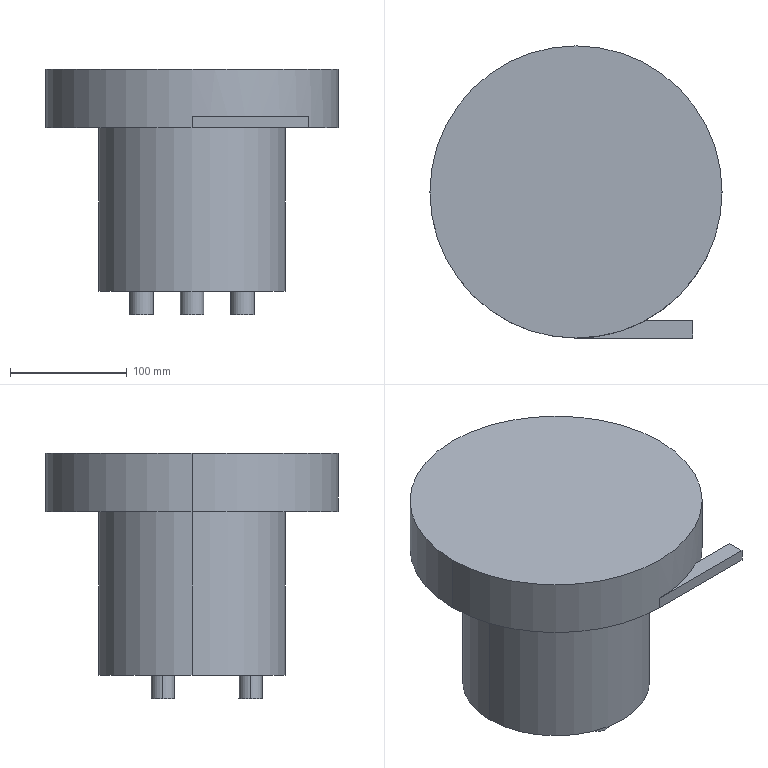Part | STEP file | O-ring vibration plate | 1 solid | 20 faces | box 250 x 250 x 210 mm | volume 5297074 mm3 | cylinder 10 | plane 10 | commonest cylinder face diameters 20 x6 160 x2 250 x2
STEP:
#1=CARTESIAN_POINT('',(0.,0.,0.));
#2=DIRECTION('',(0.,0.,1.));
#3=DIRECTION('',(1.,0.,0.));
#4=AXIS2_PLACEMENT_3D('',#1,#2,#3);
#5=CARTESIAN_POINT('',(33.301,25.,-20.));
#6=VERTEX_POINT('',#5);
#7=CARTESIAN_POINT('',(53.301,25.,-20.));
#8=VERTEX_POINT('',#7);
#9=CARTESIAN_POINT('',(43.301,25.,-20.));
#10=DIRECTION('',(0.,0.,-1.));
#11=DIRECTION('',(0.5,-0.866,0.));
#12=AXIS2_PLACEMENT_3D('',#9,#10,#11);
#13=CIRCLE('',#12,10.);
#14=CARTESIAN_POINT('',(43.301,25.,-20.));
#15=DIRECTION('',(0.,0.,1.));
#16=DIRECTION('',(1.,0.,0.));
#17=AXIS2_PLACEMENT_3D('',#14,#15,#16);
#18=CYLINDRICAL_SURFACE('',#17,10.);
#19=CARTESIAN_POINT('',(5.236,0.));
#20=DIRECTION('',(-1.,0.));
#21=VECTOR('',#20,1.);
#22=LINE('',#19,#21);
#23=(GEOMETRIC_REPRESENTATION_CONTEXT(2)PARAMETRIC_REPRESENTATION_CONTEXT()REPRESENTATION_CONTEXT('',''));
#24=DEFINITIONAL_REPRESENTATION('',(#22),#23);
#25=PCURVE('',#18,#24);
#26=CARTESIAN_POINT('',(43.301,25.,-20.));
#27=DIRECTION('',(0.,0.,-1.));
#28=DIRECTION('',(0.5,-0.866,0.));
#29=AXIS2_PLACEMENT_3D('',#26,#27,#28);
#30=PLANE('',#29);
#31=CARTESIAN_POINT('',(0.,0.));
#32=DIRECTION('',(1.,0.));
#33=AXIS2_PLACEMENT_2D('',#31,#32);
#34=CIRCLE('',#33,10.);
#35=(GEOMETRIC_REPRESENTATION_CONTEXT(2)PARAMETRIC_REPRESENTATION_CONTEXT()REPRESENTATION_CONTEXT('',''));
#36=DEFINITIONAL_REPRESENTATION('',(#34),#35);
#37=PCURVE('',#30,#36);
#38=SURFACE_CURVE('',#13,(#25,#37),.PCURVE_S1.);
#39=EDGE_CURVE('',#6,#8,#38,.T.);
#40=ORIENTED_EDGE('',*,*,#39,.F.);
#41=CARTESIAN_POINT('',(33.301,25.,0.));
#42=VERTEX_POINT('',#41);
#43=CARTESIAN_POINT('',(33.301,25.,-20.));
#44=DIRECTION('',(0.,0.,1.));
#45=VECTOR('',#44,1.);
#46=LINE('',#43,#45);
#47=CARTESIAN_POINT('',(3.142,0.));
#48=DIRECTION('',(0.,1.));
#49=VECTOR('',#48,1.);
#50=LINE('',#47,#49);
#51=(GEOMETRIC_REPRESENTATION_CONTEXT(2)PARAMETRIC_REPRESENTATION_CONTEXT()REPRESENTATION_CONTEXT('',''));
#52=DEFINITIONAL_REPRESENTATION('',(#50),#51);
#53=PCURVE('',#18,#52);
#54=CARTESIAN_POINT('',(43.301,25.,-20.));
#55=DIRECTION('',(0.,0.,1.));
#56=DIRECTION('',(1.,0.,0.));
#57=AXIS2_PLACEMENT_3D('',#54,#55,#56);
#58=CYLINDRICAL_SURFACE('',#57,10.);
#59=CARTESIAN_POINT('',(3.142,0.));
#60=DIRECTION('',(0.,1.));
#61=VECTOR('',#60,1.);
#62=LINE('',#59,#61);
#63=(GEOMETRIC_REPRESENTATION_CONTEXT(2)PARAMETRIC_REPRESENTATION_CONTEXT()REPRESENTATION_CONTEXT('',''));
#64=DEFINITIONAL_REPRESENTATION('',(#62),#63);
#65=PCURVE('',#58,#64);
#66=SURFACE_CURVE('',#46,(#53,#65),.PCURVE_S1.);
#67=EDGE_CURVE('',#6,#42,#66,.T.);
#68=ORIENTED_EDGE('',*,*,#67,.T.);
#69=CARTESIAN_POINT('',(53.301,25.,0.));
#70=VERTEX_POINT('',#69);
#71=CARTESIAN_POINT('',(43.301,25.,0.));
#72=DIRECTION('',(0.,0.,-1.));
#73=DIRECTION('',(1.,0.,0.));
#74=AXIS2_PLACEMENT_3D('',#71,#72,#73);
#75=CIRCLE('',#74,10.);
#76=CARTESIAN_POINT('',(6.283,20.));
#77=DIRECTION('',(-1.,0.));
#78=VECTOR('',#77,1.);
#79=LINE('',#76,#78);
#80=(GEOMETRIC_REPRESENTATION_CONTEXT(2)PARAMETRIC_REPRESENTATION_CONTEXT()REPRESENTATION_CONTEXT('',''));
#81=DEFINITIONAL_REPRESENTATION('',(#79),#80);
#82=PCURVE('',#18,#81);
#83=CARTESIAN_POINT('',(0.,0.,0.));
#84=DIRECTION('',(0.,0.,1.));
#85=DIRECTION('',(1.,0.,0.));
#86=AXIS2_PLACEMENT_3D('',#83,#84,#85);
#87=PLANE('',#86);
#88=CARTESIAN_POINT('',(53.301,25.));
#89=CARTESIAN_POINT('',(53.301,7.679));
#90=CARTESIAN_POINT('',(38.301,16.34));
#91=CARTESIAN_POINT('',(23.301,25.));
#92=CARTESIAN_POINT('',(38.301,33.66));
#93=CARTESIAN_POINT('',(53.301,42.321));
#94=CARTESIAN_POINT('',(53.301,25.));
#95=(BOUNDED_CURVE()B_SPLINE_CURVE(2,(#88,#89,#90,#91,#92,#93,#94),.UNSPECIFIED.,.T.,.F.)B_SPLINE_CURVE_WITH_KNOTS((1,2,2,2,2,1),(-2.094,0.,2.094,4.189,6.283,8.378),.UNSPECIFIED.)CURVE()GEOMETRIC_REPRESENTATION_ITEM()RATIONAL_B_SPLINE_CURVE((1.,0.5,1.,0.5,1.,0.5,1.))REPRESENTATION_ITEM(''));
#96=(GEOMETRIC_REPRESENTATION_CONTEXT(2)PARAMETRIC_REPRESENTATION_CONTEXT()REPRESENTATION_CONTEXT('',''));
#97=DEFINITIONAL_REPRESENTATION('',(#95),#96);
#98=PCURVE('',#87,#97);
#99=SURFACE_CURVE('',#75,(#82,#98),.PCURVE_S1.);
#100=EDGE_CURVE('',#42,#70,#99,.T.);
#101=ORIENTED_EDGE('',*,*,#100,.T.);
#102=CARTESIAN_POINT('',(53.301,25.,-20.));
#103=DIRECTION('',(0.,0.,1.));
#104=VECTOR('',#103,1.);
#105=LINE('',#102,#104);
#106=CARTESIAN_POINT('',(0.,0.));
#107=DIRECTION('',(0.,1.));
#108=VECTOR('',#107,1.);
#109=LINE('',#106,#108);
#110=(GEOMETRIC_REPRESENTATION_CONTEXT(2)PARAMETRIC_REPRESENTATION_CONTEXT()REPRESENTATION_CONTEXT('',''));
#111=DEFINITIONAL_REPRESENTATION('',(#109),#110);
#112=PCURVE('',#18,#111);
#113=CARTESIAN_POINT('',(6.283,0.));
#114=DIRECTION('',(0.,1.));
#115=VECTOR('',#114,1.);
#116=LINE('',#113,#115);
#117=(GEOMETRIC_REPRESENTATION_CONTEXT(2)PARAMETRIC_REPRESENTATION_CONTEXT()REPRESENTATION_CONTEXT('',''));
#118=DEFINITIONAL_REPRESENTATION('',(#116),#117);
#119=PCURVE('',#58,#118);
#120=SURFACE_CURVE('',#105,(#112,#119),.PCURVE_S1.);
#121=EDGE_CURVE('',#8,#70,#120,.T.);
#122=ORIENTED_EDGE('',*,*,#121,.F.);
#123=EDGE_LOOP('',(#40,#68,#101,#122));
#124=FACE_BOUND('',#123,.T.);
#125=ADVANCED_FACE('',(#124),#18,.T.);
#126=CARTESIAN_POINT('',(-53.301,25.,-20.));
#127=VERTEX_POINT('',#126);
#128=CARTESIAN_POINT('',(-33.301,25.,-20.));
#129=VERTEX_POINT('',#128);
#130=CARTESIAN_POINT('',(-43.301,25.,-20.));
#131=DIRECTION('',(0.,0.,-1.));
#132=DIRECTION('',(0.5,0.866,0.));
#133=AXIS2_PLACEMENT_3D('',#130,#131,#132);
#134=CIRCLE('',#133,10.);
#135=CARTESIAN_POINT('',(-43.301,25.,-20.));
#136=DIRECTION('',(0.,0.,1.));
#137=DIRECTION('',(1.,0.,0.));
#138=AXIS2_PLACEMENT_3D('',#135,#136,#137);
#139=CYLINDRICAL_SURFACE('',#138,10.);
#140=CARTESIAN_POINT('',(7.33,0.));
#141=DIRECTION('',(-1.,0.));
#142=VECTOR('',#141,1.);
#143=LINE('',#140,#142);
#144=(GEOMETRIC_REPRESENTATION_CONTEXT(2)PARAMETRIC_REPRESENTATION_CONTEXT()REPRESENTATION_CONTEXT('',''));
#145=DEFINITIONAL_REPRESENTATION('',(#143),#144);
#146=PCURVE('',#139,#145);
#147=CARTESIAN_POINT('',(-43.301,25.,-20.));
#148=DIRECTION('',(0.,0.,-1.));
#149=DIRECTION('',(0.5,0.866,0.));
#150=AXIS2_PLACEMENT_3D('',#147,#148,#149);
#151=PLANE('',#150);
#152=CARTESIAN_POINT('',(0.,0.));
#153=DIRECTION('',(1.,0.));
#154=AXIS2_PLACEMENT_2D('',#152,#153);
#155=CIRCLE('',#154,10.);
#156=(GEOMETRIC_REPRESENTATION_CONTEXT(2)PARAMETRIC_REPRESENTATION_CONTEXT()REPRESENTATION_CONTEXT('',''));
#157=DEFINITIONAL_REPRESENTATION('',(#155),#156);
#158=PCURVE('',#151,#157);
#159=SURFACE_CURVE('',#134,(#146,#158),.PCURVE_S1.);
#160=EDGE_CURVE('',#127,#129,#159,.T.);
#161=ORIENTED_EDGE('',*,*,#160,.F.);
#162=CARTESIAN_POINT('',(-53.301,25.,0.));
#163=VERTEX_POINT('',#162);
#164=CARTESIAN_POINT('',(-53.301,25.,-20.));
#165=DIRECTION('',(0.,0.,1.));
#166=VECTOR('',#165,1.);
#167=LINE('',#164,#166);
#168=CARTESIAN_POINT('',(3.142,0.));
#169=DIRECTION('',(0.,1.));
#170=VECTOR('',#169,1.);
#171=LINE('',#168,#170);
#172=(GEOMETRIC_REPRESENTATION_CONTEXT(2)PARAMETRIC_REPRESENTATION_CONTEXT()REPRESENTATION_CONTEXT('',''));
#173=DEFINITIONAL_REPRESENTATION('',(#171),#172);
#174=PCURVE('',#139,#173);
#175=CARTESIAN_POINT('',(-43.301,25.,-20.));
#176=DIRECTION('',(0.,0.,1.));
#177=DIRECTION('',(1.,0.,0.));
#178=AXIS2_PLACEMENT_3D('',#175,#176,#177);
#179=CYLINDRICAL_SURFACE('',#178,10.);
#180=CARTESIAN_POINT('',(3.142,0.));
#181=DIRECTION('',(0.,1.));
#182=VECTOR('',#181,1.);
#183=LINE('',#180,#182);
#184=(GEOMETRIC_REPRESENTATION_CONTEXT(2)PARAMETRIC_REPRESENTATION_CONTEXT()REPRESENTATION_CONTEXT('',''));
#185=DEFINITIONAL_REPRESENTATION('',(#183),#184);
#186=PCURVE('',#179,#185);
#187=SURFACE_CURVE('',#167,(#174,#186),.PCURVE_S1.);
#188=EDGE_CURVE('',#127,#163,#187,.T.);
#189=ORIENTED_EDGE('',*,*,#188,.T.);
#190=CARTESIAN_POINT('',(-33.301,25.,0.));
#191=VERTEX_POINT('',#190);
#192=CARTESIAN_POINT('',(-43.301,25.,0.));
#193=DIRECTION('',(0.,0.,-1.));
#194=DIRECTION('',(1.,0.,0.));
#195=AXIS2_PLACEMENT_3D('',#192,#193,#194);
#196=CIRCLE('',#195,10.);
#197=CARTESIAN_POINT('',(6.283,20.));
#198=DIRECTION('',(-1.,0.));
#199=VECTOR('',#198,1.);
#200=LINE('',#197,#199);
#201=(GEOMETRIC_REPRESENTATION_CONTEXT(2)PARAMETRIC_REPRESENTATION_CONTEXT()REPRESENTATION_CONTEXT('',''));
#202=DEFINITIONAL_REPRESENTATION('',(#200),#201);
#203=PCURVE('',#139,#202);
#204=CARTESIAN_POINT('',(-33.301,25.));
#205=CARTESIAN_POINT('',(-33.301,7.679));
#206=CARTESIAN_POINT('',(-48.301,16.34));
#207=CARTESIAN_POINT('',(-63.301,25.));
#208=CARTESIAN_POINT('',(-48.301,33.66));
#209=CARTESIAN_POINT('',(-33.301,42.321));
#210=CARTESIAN_POINT('',(-33.301,25.));
#211=(BOUNDED_CURVE()B_SPLINE_CURVE(2,(#204,#205,#206,#207,#208,#209,#210),.UNSPECIFIED.,.T.,.F.)B_SPLINE_CURVE_WITH_KNOTS((1,2,2,2,2,1),(-2.094,0.,2.094,4.189,6.283,8.378),.UNSPECIFIED.)CURVE()GEOMETRIC_REPRESENTATION_ITEM()RATIONAL_B_SPLINE_CURVE((1.,0.5,1.,0.5,1.,0.5,1.))REPRESENTATION_ITEM(''));
#212=(GEOMETRIC_REPRESENTATION_CONTEXT(2)PARAMETRIC_REPRESENTATION_CONTEXT()REPRESENTATION_CONTEXT('',''));
#213=DEFINITIONAL_REPRESENTATION('',(#211),#212);
#214=PCURVE('',#87,#213);
#215=SURFACE_CURVE('',#196,(#203,#214),.PCURVE_S1.);
#216=EDGE_CURVE('',#163,#191,#215,.T.);
#217=ORIENTED_EDGE('',*,*,#216,.T.);
#218=CARTESIAN_POINT('',(-33.301,25.,-20.));
#219=DIRECTION('',(0.,0.,1.));
#220=VECTOR('',#219,1.);
#221=LINE('',#218,#220);
#222=CARTESIAN_POINT('',(0.,0.));
#223=DIRECTION('',(0.,1.));
#224=VECTOR('',#223,1.);
#225=LINE('',#222,#224);
#226=(GEOMETRIC_REPRESENTATION_CONTEXT(2)PARAMETRIC_REPRESENTATION_CONTEXT()REPRESENTATION_CONTEXT('',''));
#227=DEFINITIONAL_REPRESENTATION('',(#225),#226);
#228=PCURVE('',#139,#227);
#229=CARTESIAN_POINT('',(6.283,0.));
#230=DIRECTION('',(0.,1.));
#231=VECTOR('',#230,1.);
#232=LINE('',#229,#231);
#233=(GEOMETRIC_REPRESENTATION_CONTEXT(2)PARAMETRIC_REPRESENTATION_CONTEXT()REPRESENTATION_CONTEXT('',''));
#234=DEFINITIONAL_REPRESENTATION('',(#232),#233);
#235=PCURVE('',#179,#234);
#236=SURFACE_CURVE('',#221,(#228,#235),.PCURVE_S1.);
#237=EDGE_CURVE('',#129,#191,#236,.T.);
#238=ORIENTED_EDGE('',*,*,#237,.F.);
#239=EDGE_LOOP('',(#161,#189,#217,#238));
#240=FACE_BOUND('',#239,.T.);
#241=ADVANCED_FACE('',(#240),#139,.T.);
#242=CARTESIAN_POINT('',(-10.,-50.,-20.));
#243=VERTEX_POINT('',#242);
#244=CARTESIAN_POINT('',(10.,-50.,-20.));
#245=VERTEX_POINT('',#244);
#246=CARTESIAN_POINT('',(0.,-50.,-20.));
#247=DIRECTION('',(0.,0.,-1.));
#248=DIRECTION('',(-1.,0.,0.));
#249=AXIS2_PLACEMENT_3D('',#246,#247,#248);
#250=CIRCLE('',#249,10.);
#251=CARTESIAN_POINT('',(0.,-50.,-20.));
#252=DIRECTION('',(0.,0.,1.));
#253=DIRECTION('',(1.,0.,0.));
#254=AXIS2_PLACEMENT_3D('',#251,#252,#253);
#255=CYLINDRICAL_SURFACE('',#254,10.);
#256=CARTESIAN_POINT('',(3.142,0.));
#257=DIRECTION('',(-1.,0.));
#258=VECTOR('',#257,1.);
#259=LINE('',#256,#258);
#260=(GEOMETRIC_REPRESENTATION_CONTEXT(2)PARAMETRIC_REPRESENTATION_CONTEXT()REPRESENTATION_CONTEXT('',''));
#261=DEFINITIONAL_REPRESENTATION('',(#259),#260);
#262=PCURVE('',#255,#261);
#263=CARTESIAN_POINT('',(0.,-50.,-20.));
#264=DIRECTION('',(0.,0.,-1.));
#265=DIRECTION('',(-1.,0.,0.));
#266=AXIS2_PLACEMENT_3D('',#263,#264,#265);
#267=PLANE('',#266);
#268=CARTESIAN_POINT('',(0.,0.));
#269=DIRECTION('',(1.,0.));
#270=AXIS2_PLACEMENT_2D('',#268,#269);
#271=CIRCLE('',#270,10.);
#272=(GEOMETRIC_REPRESENTATION_CONTEXT(2)PARAMETRIC_REPRESENTATION_CONTEXT()REPRESENTATION_CONTEXT('',''));
#273=DEFINITIONAL_REPRESENTATION('',(#271),#272);
#274=PCURVE('',#267,#273);
#275=SURFACE_CURVE('',#250,(#262,#274),.PCURVE_S1.);
#276=EDGE_CURVE('',#243,#245,#275,.T.);
#277=ORIENTED_EDGE('',*,*,#276,.F.);
#278=CARTESIAN_POINT('',(-10.,-50.,0.));
#279=VERTEX_POINT('',#278);
#280=CARTESIAN_POINT('',(-10.,-50.,-20.));
#281=DIRECTION('',(0.,0.,1.));
#282=VECTOR('',#281,1.);
#283=LINE('',#280,#282);
#284=CARTESIAN_POINT('',(3.142,0.));
#285=DIRECTION('',(0.,1.));
#286=VECTOR('',#285,1.);
#287=LINE('',#284,#286);
#288=(GEOMETRIC_REPRESENTATION_CONTEXT(2)PARAMETRIC_REPRESENTATION_CONTEXT()REPRESENTATION_CONTEXT('',''));
#289=DEFINITIONAL_REPRESENTATION('',(#287),#288);
#290=PCURVE('',#255,#289);
#291=CARTESIAN_POINT('',(0.,-50.,-20.));
#292=DIRECTION('',(0.,0.,1.));
#293=DIRECTION('',(1.,0.,0.));
#294=AXIS2_PLACEMENT_3D('',#291,#292,#293);
#295=CYLINDRICAL_SURFACE('',#294,10.);
#296=CARTESIAN_POINT('',(3.142,0.));
#297=DIRECTION('',(0.,1.));
#298=VECTOR('',#297,1.);
#299=LINE('',#296,#298);
#300=(GEOMETRIC_REPRESENTATION_CONTEXT(2)PARAMETRIC_REPRESENTATION_CONTEXT()REPRESENTATION_CONTEXT('',''));
#301=DEFINITIONAL_REPRESENTATION('',(#299),#300);
#302=PCURVE('',#295,#301);
#303=SURFACE_CURVE('',#283,(#290,#302),.PCURVE_S1.);
#304=EDGE_CURVE('',#243,#279,#303,.T.);
#305=ORIENTED_EDGE('',*,*,#304,.T.);
#306=CARTESIAN_POINT('',(10.,-50.,0.));
#307=VERTEX_POINT('',#306);
#308=CARTESIAN_POINT('',(0.,-50.,0.));
#309=DIRECTION('',(0.,0.,-1.));
#310=DIRECTION('',(1.,0.,0.));
#311=AXIS2_PLACEMENT_3D('',#308,#309,#310);
#312=CIRCLE('',#311,10.);
#313=CARTESIAN_POINT('',(6.283,20.));
#314=DIRECTION('',(-1.,0.));
#315=VECTOR('',#314,1.);
#316=LINE('',#313,#315);
#317=(GEOMETRIC_REPRESENTATION_CONTEXT(2)PARAMETRIC_REPRESENTATION_CONTEXT()REPRESENTATION_CONTEXT('',''));
#318=DEFINITIONAL_REPRESENTATION('',(#316),#317);
#319=PCURVE('',#255,#318);
#320=CARTESIAN_POINT('',(10.,-50.));
#321=CARTESIAN_POINT('',(10.,-67.321));
#322=CARTESIAN_POINT('',(-5.,-58.66));
#323=CARTESIAN_POINT('',(-20.,-50.));
#324=CARTESIAN_POINT('',(-5.,-41.34));
#325=CARTESIAN_POINT('',(10.,-32.679));
#326=CARTESIAN_POINT('',(10.,-50.));
#327=(BOUNDED_CURVE()B_SPLINE_CURVE(2,(#320,#321,#322,#323,#324,#325,#326),.UNSPECIFIED.,.T.,.F.)B_SPLINE_CURVE_WITH_KNOTS((1,2,2,2,2,1),(-2.094,0.,2.094,4.189,6.283,8.378),.UNSPECIFIED.)CURVE()GEOMETRIC_REPRESENTATION_ITEM()RATIONAL_B_SPLINE_CURVE((1.,0.5,1.,0.5,1.,0.5,1.))REPRESENTATION_ITEM(''));
#328=(GEOMETRIC_REPRESENTATION_CONTEXT(2)PARAMETRIC_REPRESENTATION_CONTEXT()REPRESENTATION_CONTEXT('',''));
#329=DEFINITIONAL_REPRESENTATION('',(#327),#328);
#330=PCURVE('',#87,#329);
#331=SURFACE_CURVE('',#312,(#319,#330),.PCURVE_S1.);
#332=EDGE_CURVE('',#279,#307,#331,.T.);
#333=ORIENTED_EDGE('',*,*,#332,.T.);
#334=CARTESIAN_POINT('',(10.,-50.,-20.));
#335=DIRECTION('',(0.,0.,1.));
#336=VECTOR('',#335,1.);
#337=LINE('',#334,#336);
#338=CARTESIAN_POINT('',(0.,0.));
#339=DIRECTION('',(0.,1.));
#340=VECTOR('',#339,1.);
#341=LINE('',#338,#340);
#342=(GEOMETRIC_REPRESENTATION_CONTEXT(2)PARAMETRIC_REPRESENTATION_CONTEXT()REPRESENTATION_CONTEXT('',''));
#343=DEFINITIONAL_REPRESENTATION('',(#341),#342);
#344=PCURVE('',#255,#343);
#345=CARTESIAN_POINT('',(6.283,0.));
#346=DIRECTION('',(0.,1.));
#347=VECTOR('',#346,1.);
#348=LINE('',#345,#347);
#349=(GEOMETRIC_REPRESENTATION_CONTEXT(2)PARAMETRIC_REPRESENTATION_CONTEXT()REPRESENTATION_CONTEXT('',''));
#350=DEFINITIONAL_REPRESENTATION('',(#348),#349);
#351=PCURVE('',#295,#350);
#352=SURFACE_CURVE('',#337,(#344,#351),.PCURVE_S1.);
#353=EDGE_CURVE('',#245,#307,#352,.T.);
#354=ORIENTED_EDGE('',*,*,#353,.F.);
#355=EDGE_LOOP('',(#277,#305,#333,#354));
#356=FACE_BOUND('',#355,.T.);
#357=ADVANCED_FACE('',(#356),#255,.T.);
#358=CARTESIAN_POINT('',(80.,0.,140.));
#359=VERTEX_POINT('',#358);
#360=CARTESIAN_POINT('',(-80.,0.,140.));
#361=VERTEX_POINT('',#360);
#362=CARTESIAN_POINT('',(0.,0.,140.));
#363=DIRECTION('',(0.,0.,1.));
#364=DIRECTION('',(1.,0.,0.));
#365=AXIS2_PLACEMENT_3D('',#362,#363,#364);
#366=CIRCLE('',#365,80.);
#367=CARTESIAN_POINT('',(0.,0.,140.));
#368=DIRECTION('',(0.,0.,-1.));
#369=DIRECTION('',(-1.,0.,0.));
#370=AXIS2_PLACEMENT_3D('',#367,#368,#369);
#371=CYLINDRICAL_SURFACE('',#370,80.);
#372=CARTESIAN_POINT('',(3.142,0.));
#373=DIRECTION('',(-1.,0.));
#374=VECTOR('',#373,1.);
#375=LINE('',#372,#374);
#376=(GEOMETRIC_REPRESENTATION_CONTEXT(2)PARAMETRIC_REPRESENTATION_CONTEXT()REPRESENTATION_CONTEXT('',''));
#377=DEFINITIONAL_REPRESENTATION('',(#375),#376);
#378=PCURVE('',#371,#377);
#379=CARTESIAN_POINT('',(0.,0.,140.));
#380=DIRECTION('',(0.,0.,1.));
#381=DIRECTION('',(1.,0.,0.));
#382=AXIS2_PLACEMENT_3D('',#379,#380,#381);
#383=PLANE('',#382);
#384=CARTESIAN_POINT('',(0.,0.));
#385=DIRECTION('',(1.,0.));
#386=AXIS2_PLACEMENT_2D('',#384,#385);
#387=CIRCLE('',#386,80.);
#388=(GEOMETRIC_REPRESENTATION_CONTEXT(2)PARAMETRIC_REPRESENTATION_CONTEXT()REPRESENTATION_CONTEXT('',''));
#389=DEFINITIONAL_REPRESENTATION('',(#387),#388);
#390=PCURVE('',#383,#389);
#391=SURFACE_CURVE('',#366,(#378,#390),.PCURVE_S1.);
#392=EDGE_CURVE('',#359,#361,#391,.T.);
#393=ORIENTED_EDGE('',*,*,#392,.F.);
#394=CARTESIAN_POINT('',(80.,0.,0.));
#395=VERTEX_POINT('',#394);
#396=CARTESIAN_POINT('',(80.,0.,140.));
#397=DIRECTION('',(0.,0.,-1.));
#398=VECTOR('',#397,1.);
#399=LINE('',#396,#398);
#400=CARTESIAN_POINT('',(3.142,0.));
#401=DIRECTION('',(0.,1.));
#402=VECTOR('',#401,1.);
#403=LINE('',#400,#402);
#404=(GEOMETRIC_REPRESENTATION_CONTEXT(2)PARAMETRIC_REPRESENTATION_CONTEXT()REPRESENTATION_CONTEXT('',''));
#405=DEFINITIONAL_REPRESENTATION('',(#403),#404);
#406=PCURVE('',#371,#405);
#407=CARTESIAN_POINT('',(0.,0.,140.));
#408=DIRECTION('',(0.,0.,-1.));
#409=DIRECTION('',(-1.,0.,0.));
#410=AXIS2_PLACEMENT_3D('',#407,#408,#409);
#411=CYLINDRICAL_SURFACE('',#410,80.);
#412=CARTESIAN_POINT('',(3.142,0.));
#413=DIRECTION('',(0.,1.));
#414=VECTOR('',#413,1.);
#415=LINE('',#412,#414);
#416=(GEOMETRIC_REPRESENTATION_CONTEXT(2)PARAMETRIC_REPRESENTATION_CONTEXT()REPRESENTATION_CONTEXT('',''));
#417=DEFINITIONAL_REPRESENTATION('',(#415),#416);
#418=PCURVE('',#411,#417);
#419=SURFACE_CURVE('',#399,(#406,#418),.PCURVE_S1.);
#420=EDGE_CURVE('',#359,#395,#419,.T.);
#421=ORIENTED_EDGE('',*,*,#420,.T.);
#422=CARTESIAN_POINT('',(-80.,0.,0.));
#423=VERTEX_POINT('',#422);
#424=CARTESIAN_POINT('',(0.,0.,0.));
#425=DIRECTION('',(0.,0.,1.));
#426=DIRECTION('',(1.,0.,0.));
#427=AXIS2_PLACEMENT_3D('',#424,#425,#426);
#428=CIRCLE('',#427,80.);
#429=CARTESIAN_POINT('',(3.142,140.));
#430=DIRECTION('',(-1.,0.));
#431=VECTOR('',#430,1.);
#432=LINE('',#429,#431);
#433=(GEOMETRIC_REPRESENTATION_CONTEXT(2)PARAMETRIC_REPRESENTATION_CONTEXT()REPRESENTATION_CONTEXT('',''));
#434=DEFINITIONAL_REPRESENTATION('',(#432),#433);
#435=PCURVE('',#371,#434);
#436=CARTESIAN_POINT('',(0.,0.));
#437=DIRECTION('',(1.,0.));
#438=AXIS2_PLACEMENT_2D('',#436,#437);
#439=CIRCLE('',#438,80.);
#440=(GEOMETRIC_REPRESENTATION_CONTEXT(2)PARAMETRIC_REPRESENTATION_CONTEXT()REPRESENTATION_CONTEXT('',''));
#441=DEFINITIONAL_REPRESENTATION('',(#439),#440);
#442=PCURVE('',#87,#441);
#443=SURFACE_CURVE('',#428,(#435,#442),.PCURVE_S1.);
#444=EDGE_CURVE('',#395,#423,#443,.T.);
#445=ORIENTED_EDGE('',*,*,#444,.T.);
#446=CARTESIAN_POINT('',(-80.,0.,140.));
#447=DIRECTION('',(0.,0.,-1.));
#448=VECTOR('',#447,1.);
#449=LINE('',#446,#448);
#450=CARTESIAN_POINT('',(0.,0.));
#451=DIRECTION('',(0.,1.));
#452=VECTOR('',#451,1.);
#453=LINE('',#450,#452);
#454=(GEOMETRIC_REPRESENTATION_CONTEXT(2)PARAMETRIC_REPRESENTATION_CONTEXT()REPRESENTATION_CONTEXT('',''));
#455=DEFINITIONAL_REPRESENTATION('',(#453),#454);
#456=PCURVE('',#371,#455);
#457=CARTESIAN_POINT('',(6.283,0.));
#458=DIRECTION('',(0.,1.));
#459=VECTOR('',#458,1.);
#460=LINE('',#457,#459);
#461=(GEOMETRIC_REPRESENTATION_CONTEXT(2)PARAMETRIC_REPRESENTATION_CONTEXT()REPRESENTATION_CONTEXT('',''));
#462=DEFINITIONAL_REPRESENTATION('',(#460),#461);
#463=PCURVE('',#411,#462);
#464=SURFACE_CURVE('',#449,(#456,#463),.PCURVE_S1.);
#465=EDGE_CURVE('',#361,#423,#464,.T.);
#466=ORIENTED_EDGE('',*,*,#465,.F.);
#467=EDGE_LOOP('',(#393,#421,#445,#466));
#468=FACE_BOUND('',#467,.T.);
#469=ADVANCED_FACE('',(#468),#371,.T.);
#470=CARTESIAN_POINT('',(125.,0.,190.));
#471=VERTEX_POINT('',#470);
#472=CARTESIAN_POINT('',(-125.,0.,190.));
#473=VERTEX_POINT('',#472);
#474=CARTESIAN_POINT('',(0.,0.,190.));
#475=DIRECTION('',(0.,0.,1.));
#476=DIRECTION('',(1.,0.,0.));
#477=AXIS2_PLACEMENT_3D('',#474,#475,#476);
#478=CIRCLE('',#477,125.);
#479=CARTESIAN_POINT('',(0.,0.,190.));
#480=DIRECTION('',(0.,0.,-1.));
#481=DIRECTION('',(-1.,0.,0.));
#482=AXIS2_PLACEMENT_3D('',#479,#480,#481);
#483=CYLINDRICAL_SURFACE('',#482,125.);
#484=CARTESIAN_POINT('',(3.142,0.));
#485=DIRECTION('',(-1.,0.));
#486=VECTOR('',#485,1.);
#487=LINE('',#484,#486);
#488=(GEOMETRIC_REPRESENTATION_CONTEXT(2)PARAMETRIC_REPRESENTATION_CONTEXT()REPRESENTATION_CONTEXT('',''));
#489=DEFINITIONAL_REPRESENTATION('',(#487),#488);
#490=PCURVE('',#483,#489);
#491=CARTESIAN_POINT('',(0.,0.,190.));
#492=DIRECTION('',(0.,0.,1.));
#493=DIRECTION('',(1.,0.,0.));
#494=AXIS2_PLACEMENT_3D('',#491,#492,#493);
#495=PLANE('',#494);
#496=CARTESIAN_POINT('',(0.,0.));
#497=DIRECTION('',(1.,0.));
#498=AXIS2_PLACEMENT_2D('',#496,#497);
#499=CIRCLE('',#498,125.);
#500=(GEOMETRIC_REPRESENTATION_CONTEXT(2)PARAMETRIC_REPRESENTATION_CONTEXT()REPRESENTATION_CONTEXT('',''));
#501=DEFINITIONAL_REPRESENTATION('',(#499),#500);
#502=PCURVE('',#495,#501);
#503=SURFACE_CURVE('',#478,(#490,#502),.PCURVE_S1.);
#504=EDGE_CURVE('',#471,#473,#503,.T.);
#505=ORIENTED_EDGE('',*,*,#504,.F.);
#506=CARTESIAN_POINT('',(125.,0.,140.));
#507=VERTEX_POINT('',#506);
#508=CARTESIAN_POINT('',(125.,0.,190.));
#509=DIRECTION('',(0.,0.,-1.));
#510=VECTOR('',#509,1.);
#511=LINE('',#508,#510);
#512=CARTESIAN_POINT('',(3.142,0.));
#513=DIRECTION('',(0.,1.));
#514=VECTOR('',#513,1.);
#515=LINE('',#512,#514);
#516=(GEOMETRIC_REPRESENTATION_CONTEXT(2)PARAMETRIC_REPRESENTATION_CONTEXT()REPRESENTATION_CONTEXT('',''));
#517=DEFINITIONAL_REPRESENTATION('',(#515),#516);
#518=PCURVE('',#483,#517);
#519=CARTESIAN_POINT('',(0.,0.,190.));
#520=DIRECTION('',(0.,0.,-1.));
#521=DIRECTION('',(-1.,0.,0.));
#522=AXIS2_PLACEMENT_3D('',#519,#520,#521);
#523=CYLINDRICAL_SURFACE('',#522,125.);
#524=CARTESIAN_POINT('',(3.142,0.));
#525=DIRECTION('',(0.,1.));
#526=VECTOR('',#525,1.);
#527=LINE('',#524,#526);
#528=(GEOMETRIC_REPRESENTATION_CONTEXT(2)PARAMETRIC_REPRESENTATION_CONTEXT()REPRESENTATION_CONTEXT('',''));
#529=DEFINITIONAL_REPRESENTATION('',(#527),#528);
#530=PCURVE('',#523,#529);
#531=SURFACE_CURVE('',#511,(#518,#530),.PCURVE_S1.);
#532=EDGE_CURVE('',#471,#507,#531,.T.);
#533=ORIENTED_EDGE('',*,*,#532,.T.);
#534=CARTESIAN_POINT('',(-125.,0.,140.));
#535=VERTEX_POINT('',#534);
#536=CARTESIAN_POINT('',(0.,0.,140.));
#537=DIRECTION('',(0.,0.,1.));
#538=DIRECTION('',(1.,0.,0.));
#539=AXIS2_PLACEMENT_3D('',#536,#537,#538);
#540=CIRCLE('',#539,125.);
#541=CARTESIAN_POINT('',(3.142,50.));
#542=DIRECTION('',(-1.,0.));
#543=VECTOR('',#542,1.);
#544=LINE('',#541,#543);
#545=(GEOMETRIC_REPRESENTATION_CONTEXT(2)PARAMETRIC_REPRESENTATION_CONTEXT()REPRESENTATION_CONTEXT('',''));
#546=DEFINITIONAL_REPRESENTATION('',(#544),#545);
#547=PCURVE('',#483,#546);
#548=CARTESIAN_POINT('',(0.,0.));
#549=DIRECTION('',(1.,0.));
#550=AXIS2_PLACEMENT_2D('',#548,#549);
#551=CIRCLE('',#550,125.);
#552=(GEOMETRIC_REPRESENTATION_CONTEXT(2)PARAMETRIC_REPRESENTATION_CONTEXT()REPRESENTATION_CONTEXT('',''));
#553=DEFINITIONAL_REPRESENTATION('',(#551),#552);
#554=PCURVE('',#383,#553);
#555=SURFACE_CURVE('',#540,(#547,#554),.PCURVE_S1.);
#556=EDGE_CURVE('',#507,#535,#555,.T.);
#557=ORIENTED_EDGE('',*,*,#556,.T.);
#558=CARTESIAN_POINT('',(-125.,0.,190.));
#559=DIRECTION('',(0.,0.,-1.));
#560=VECTOR('',#559,1.);
#561=LINE('',#558,#560);
#562=CARTESIAN_POINT('',(0.,0.));
#563=DIRECTION('',(0.,1.));
#564=VECTOR('',#563,1.);
#565=LINE('',#562,#564);
#566=(GEOMETRIC_REPRESENTATION_CONTEXT(2)PARAMETRIC_REPRESENTATION_CONTEXT()REPRESENTATION_CONTEXT('',''));
#567=DEFINITIONAL_REPRESENTATION('',(#565),#566);
#568=PCURVE('',#483,#567);
#569=CARTESIAN_POINT('',(6.283,0.));
#570=DIRECTION('',(0.,1.));
#571=VECTOR('',#570,1.);
#572=LINE('',#569,#571);
#573=(GEOMETRIC_REPRESENTATION_CONTEXT(2)PARAMETRIC_REPRESENTATION_CONTEXT()REPRESENTATION_CONTEXT('',''));
#574=DEFINITIONAL_REPRESENTATION('',(#572),#573);
#575=PCURVE('',#523,#574);
#576=SURFACE_CURVE('',#561,(#568,#575),.PCURVE_S1.);
#577=EDGE_CURVE('',#473,#535,#576,.T.);
#578=ORIENTED_EDGE('',*,*,#577,.F.);
#579=EDGE_LOOP('',(#505,#533,#557,#578));
#580=FACE_BOUND('',#579,.T.);
#581=ADVANCED_FACE('',(#580),#483,.T.);
#582=CARTESIAN_POINT('',(-43.301,25.,0.));
#583=DIRECTION('',(0.,0.,-1.));
#584=DIRECTION('',(1.,0.,0.));
#585=AXIS2_PLACEMENT_3D('',#582,#583,#584);
#586=CIRCLE('',#585,10.);
#587=CARTESIAN_POINT('',(-33.301,25.));
#588=CARTESIAN_POINT('',(-33.301,7.679));
#589=CARTESIAN_POINT('',(-48.301,16.34));
#590=CARTESIAN_POINT('',(-63.301,25.));
#591=CARTESIAN_POINT('',(-48.301,33.66));
#592=CARTESIAN_POINT('',(-33.301,42.321));
#593=CARTESIAN_POINT('',(-33.301,25.));
#594=(BOUNDED_CURVE()B_SPLINE_CURVE(2,(#587,#588,#589,#590,#591,#592,#593),.UNSPECIFIED.,.T.,.F.)B_SPLINE_CURVE_WITH_KNOTS((1,2,2,2,2,1),(-2.094,0.,2.094,4.189,6.283,8.378),.UNSPECIFIED.)CURVE()GEOMETRIC_REPRESENTATION_ITEM()RATIONAL_B_SPLINE_CURVE((1.,0.5,1.,0.5,1.,0.5,1.))REPRESENTATION_ITEM(''));
#595=(GEOMETRIC_REPRESENTATION_CONTEXT(2)PARAMETRIC_REPRESENTATION_CONTEXT()REPRESENTATION_CONTEXT('',''));
#596=DEFINITIONAL_REPRESENTATION('',(#594),#595);
#597=PCURVE('',#87,#596);
#598=CARTESIAN_POINT('',(6.283,20.));
#599=DIRECTION('',(-1.,0.));
#600=VECTOR('',#599,1.);
#601=LINE('',#598,#600);
#602=(GEOMETRIC_REPRESENTATION_CONTEXT(2)PARAMETRIC_REPRESENTATION_CONTEXT()REPRESENTATION_CONTEXT('',''));
#603=DEFINITIONAL_REPRESENTATION('',(#601),#602);
#604=PCURVE('',#179,#603);
#605=SURFACE_CURVE('',#586,(#597,#604),.PCURVE_S1.);
#606=EDGE_CURVE('',#191,#163,#605,.T.);
#607=ORIENTED_EDGE('',*,*,#606,.F.);
#608=ORIENTED_EDGE('',*,*,#216,.F.);
#609=EDGE_LOOP('',(#607,#608));
#610=FACE_BOUND('',#609,.T.);
#611=CARTESIAN_POINT('',(0.,0.,0.));
#612=DIRECTION('',(0.,0.,1.));
#613=DIRECTION('',(1.,0.,0.));
#614=AXIS2_PLACEMENT_3D('',#611,#612,#613);
#615=CIRCLE('',#614,80.);
#616=CARTESIAN_POINT('',(0.,0.));
#617=DIRECTION('',(1.,0.));
#618=AXIS2_PLACEMENT_2D('',#616,#617);
#619=CIRCLE('',#618,80.);
#620=(GEOMETRIC_REPRESENTATION_CONTEXT(2)PARAMETRIC_REPRESENTATION_CONTEXT()REPRESENTATION_CONTEXT('',''));
#621=DEFINITIONAL_REPRESENTATION('',(#619),#620);
#622=PCURVE('',#87,#621);
#623=CARTESIAN_POINT('',(9.425,140.));
#624=DIRECTION('',(-1.,0.));
#625=VECTOR('',#624,1.);
#626=LINE('',#623,#625);
#627=(GEOMETRIC_REPRESENTATION_CONTEXT(2)PARAMETRIC_REPRESENTATION_CONTEXT()REPRESENTATION_CONTEXT('',''));
#628=DEFINITIONAL_REPRESENTATION('',(#626),#627);
#629=PCURVE('',#411,#628);
#630=SURFACE_CURVE('',#615,(#622,#629),.PCURVE_S1.);
#631=EDGE_CURVE('',#423,#395,#630,.T.);
#632=ORIENTED_EDGE('',*,*,#631,.F.);
#633=ORIENTED_EDGE('',*,*,#444,.F.);
#634=EDGE_LOOP('',(#632,#633));
#635=FACE_BOUND('',#634,.T.);
#636=CARTESIAN_POINT('',(0.,-50.,0.));
#637=DIRECTION('',(0.,0.,-1.));
#638=DIRECTION('',(1.,0.,0.));
#639=AXIS2_PLACEMENT_3D('',#636,#637,#638);
#640=CIRCLE('',#639,10.);
#641=CARTESIAN_POINT('',(10.,-50.));
#642=CARTESIAN_POINT('',(10.,-67.321));
#643=CARTESIAN_POINT('',(-5.,-58.66));
#644=CARTESIAN_POINT('',(-20.,-50.));
#645=CARTESIAN_POINT('',(-5.,-41.34));
#646=CARTESIAN_POINT('',(10.,-32.679));
#647=CARTESIAN_POINT('',(10.,-50.));
#648=(BOUNDED_CURVE()B_SPLINE_CURVE(2,(#641,#642,#643,#644,#645,#646,#647),.UNSPECIFIED.,.T.,.F.)B_SPLINE_CURVE_WITH_KNOTS((1,2,2,2,2,1),(-2.094,0.,2.094,4.189,6.283,8.378),.UNSPECIFIED.)CURVE()GEOMETRIC_REPRESENTATION_ITEM()RATIONAL_B_SPLINE_CURVE((1.,0.5,1.,0.5,1.,0.5,1.))REPRESENTATION_ITEM(''));
#649=(GEOMETRIC_REPRESENTATION_CONTEXT(2)PARAMETRIC_REPRESENTATION_CONTEXT()REPRESENTATION_CONTEXT('',''));
#650=DEFINITIONAL_REPRESENTATION('',(#648),#649);
#651=PCURVE('',#87,#650);
#652=CARTESIAN_POINT('',(6.283,20.));
#653=DIRECTION('',(-1.,0.));
#654=VECTOR('',#653,1.);
#655=LINE('',#652,#654);
#656=(GEOMETRIC_REPRESENTATION_CONTEXT(2)PARAMETRIC_REPRESENTATION_CONTEXT()REPRESENTATION_CONTEXT('',''));
#657=DEFINITIONAL_REPRESENTATION('',(#655),#656);
#658=PCURVE('',#295,#657);
#659=SURFACE_CURVE('',#640,(#651,#658),.PCURVE_S1.);
#660=EDGE_CURVE('',#307,#279,#659,.T.);
#661=ORIENTED_EDGE('',*,*,#660,.F.);
#662=ORIENTED_EDGE('',*,*,#332,.F.);
#663=EDGE_LOOP('',(#661,#662));
#664=FACE_BOUND('',#663,.T.);
#665=CARTESIAN_POINT('',(43.301,25.,0.));
#666=DIRECTION('',(0.,0.,-1.));
#667=DIRECTION('',(1.,0.,0.));
#668=AXIS2_PLACEMENT_3D('',#665,#666,#667);
#669=CIRCLE('',#668,10.);
#670=CARTESIAN_POINT('',(53.301,25.));
#671=CARTESIAN_POINT('',(53.301,7.679));
#672=CARTESIAN_POINT('',(38.301,16.34));
#673=CARTESIAN_POINT('',(23.301,25.));
#674=CARTESIAN_POINT('',(38.301,33.66));
#675=CARTESIAN_POINT('',(53.301,42.321));
#676=CARTESIAN_POINT('',(53.301,25.));
#677=(BOUNDED_CURVE()B_SPLINE_CURVE(2,(#670,#671,#672,#673,#674,#675,#676),.UNSPECIFIED.,.T.,.F.)B_SPLINE_CURVE_WITH_KNOTS((1,2,2,2,2,1),(-2.094,0.,2.094,4.189,6.283,8.378),.UNSPECIFIED.)CURVE()GEOMETRIC_REPRESENTATION_ITEM()RATIONAL_B_SPLINE_CURVE((1.,0.5,1.,0.5,1.,0.5,1.))REPRESENTATION_ITEM(''));
#678=(GEOMETRIC_REPRESENTATION_CONTEXT(2)PARAMETRIC_REPRESENTATION_CONTEXT()REPRESENTATION_CONTEXT('',''));
#679=DEFINITIONAL_REPRESENTATION('',(#677),#678);
#680=PCURVE('',#87,#679);
#681=CARTESIAN_POINT('',(6.283,20.));
#682=DIRECTION('',(-1.,0.));
#683=VECTOR('',#682,1.);
#684=LINE('',#681,#683);
#685=(GEOMETRIC_REPRESENTATION_CONTEXT(2)PARAMETRIC_REPRESENTATION_CONTEXT()REPRESENTATION_CONTEXT('',''));
#686=DEFINITIONAL_REPRESENTATION('',(#684),#685);
#687=PCURVE('',#58,#686);
#688=SURFACE_CURVE('',#669,(#680,#687),.PCURVE_S1.);
#689=EDGE_CURVE('',#70,#42,#688,.T.);
#690=ORIENTED_EDGE('',*,*,#689,.F.);
#691=ORIENTED_EDGE('',*,*,#100,.F.);
#692=EDGE_LOOP('',(#690,#691));
#693=FACE_BOUND('',#692,.T.);
#694=ADVANCED_FACE('',(#610,#635,#664,#693),#87,.F.);
#695=ORIENTED_EDGE('',*,*,#532,.F.);
#696=CARTESIAN_POINT('',(0.,0.,190.));
#697=DIRECTION('',(0.,0.,1.));
#698=DIRECTION('',(1.,0.,0.));
#699=AXIS2_PLACEMENT_3D('',#696,#697,#698);
#700=CIRCLE('',#699,125.);
#701=CARTESIAN_POINT('',(9.425,0.));
#702=DIRECTION('',(-1.,0.));
#703=VECTOR('',#702,1.);
#704=LINE('',#701,#703);
#705=(GEOMETRIC_REPRESENTATION_CONTEXT(2)PARAMETRIC_REPRESENTATION_CONTEXT()REPRESENTATION_CONTEXT('',''));
#706=DEFINITIONAL_REPRESENTATION('',(#704),#705);
#707=PCURVE('',#523,#706);
#708=CARTESIAN_POINT('',(0.,0.));
#709=DIRECTION('',(1.,0.));
#710=AXIS2_PLACEMENT_2D('',#708,#709);
#711=CIRCLE('',#710,125.);
#712=(GEOMETRIC_REPRESENTATION_CONTEXT(2)PARAMETRIC_REPRESENTATION_CONTEXT()REPRESENTATION_CONTEXT('',''));
#713=DEFINITIONAL_REPRESENTATION('',(#711),#712);
#714=PCURVE('',#495,#713);
#715=SURFACE_CURVE('',#700,(#707,#714),.PCURVE_S1.);
#716=EDGE_CURVE('',#473,#471,#715,.T.);
#717=ORIENTED_EDGE('',*,*,#716,.F.);
#718=ORIENTED_EDGE('',*,*,#577,.T.);
#719=CARTESIAN_POINT('',(0.,-125.,140.));
#720=VERTEX_POINT('',#719);
#721=CARTESIAN_POINT('',(0.,0.,140.));
#722=DIRECTION('',(0.,0.,1.));
#723=DIRECTION('',(1.,0.,0.));
#724=AXIS2_PLACEMENT_3D('',#721,#722,#723);
#725=CIRCLE('',#724,125.);
#726=CARTESIAN_POINT('',(9.425,50.));
#727=DIRECTION('',(-1.,0.));
#728=VECTOR('',#727,1.);
#729=LINE('',#726,#728);
#730=(GEOMETRIC_REPRESENTATION_CONTEXT(2)PARAMETRIC_REPRESENTATION_CONTEXT()REPRESENTATION_CONTEXT('',''));
#731=DEFINITIONAL_REPRESENTATION('',(#729),#730);
#732=PCURVE('',#523,#731);
#733=CARTESIAN_POINT('',(0.,0.));
#734=DIRECTION('',(1.,0.));
#735=AXIS2_PLACEMENT_2D('',#733,#734);
#736=CIRCLE('',#735,125.);
#737=(GEOMETRIC_REPRESENTATION_CONTEXT(2)PARAMETRIC_REPRESENTATION_CONTEXT()REPRESENTATION_CONTEXT('',''));
#738=DEFINITIONAL_REPRESENTATION('',(#736),#737);
#739=PCURVE('',#383,#738);
#740=SURFACE_CURVE('',#725,(#732,#739),.PCURVE_S1.);
#741=EDGE_CURVE('',#535,#720,#740,.T.);
#742=ORIENTED_EDGE('',*,*,#741,.T.);
#743=CARTESIAN_POINT('',(0.,-125.,150.));
#744=VERTEX_POINT('',#743);
#745=CARTESIAN_POINT('',(0.,-125.,150.));
#746=DIRECTION('',(0.,0.,-1.));
#747=VECTOR('',#746,1.);
#748=LINE('',#745,#747);
#749=CARTESIAN_POINT('',(4.712,40.));
#750=DIRECTION('',(0.,1.));
#751=VECTOR('',#750,1.);
#752=LINE('',#749,#751);
#753=(GEOMETRIC_REPRESENTATION_CONTEXT(2)PARAMETRIC_REPRESENTATION_CONTEXT()REPRESENTATION_CONTEXT('',''));
#754=DEFINITIONAL_REPRESENTATION('',(#752),#753);
#755=PCURVE('',#523,#754);
#756=CARTESIAN_POINT('',(0.,-125.,150.));
#757=DIRECTION('',(0.,1.,0.));
#758=DIRECTION('',(0.,0.,1.));
#759=AXIS2_PLACEMENT_3D('',#756,#757,#758);
#760=PLANE('',#759);
#761=CARTESIAN_POINT('',(0.,0.));
#762=DIRECTION('',(-1.,0.));
#763=VECTOR('',#762,1.);
#764=LINE('',#761,#763);
#765=(GEOMETRIC_REPRESENTATION_CONTEXT(2)PARAMETRIC_REPRESENTATION_CONTEXT()REPRESENTATION_CONTEXT('',''));
#766=DEFINITIONAL_REPRESENTATION('',(#764),#765);
#767=PCURVE('',#760,#766);
#768=SURFACE_CURVE('',#748,(#755,#767),.PCURVE_S1.);
#769=EDGE_CURVE('',#744,#720,#768,.T.);
#770=ORIENTED_EDGE('',*,*,#769,.F.);
#771=CARTESIAN_POINT('',(59.372,-110.,150.));
#772=VERTEX_POINT('',#771);
#773=CARTESIAN_POINT('',(0.,0.,150.));
#774=DIRECTION('',(0.,0.,1.));
#775=DIRECTION('',(1.,0.,0.));
#776=AXIS2_PLACEMENT_3D('',#773,#774,#775);
#777=CIRCLE('',#776,125.);
#778=CARTESIAN_POINT('',(9.425,40.));
#779=DIRECTION('',(-1.,0.));
#780=VECTOR('',#779,1.);
#781=LINE('',#778,#780);
#782=(GEOMETRIC_REPRESENTATION_CONTEXT(2)PARAMETRIC_REPRESENTATION_CONTEXT()REPRESENTATION_CONTEXT('',''));
#783=DEFINITIONAL_REPRESENTATION('',(#781),#782);
#784=PCURVE('',#523,#783);
#785=CARTESIAN_POINT('',(0.,0.,150.));
#786=DIRECTION('',(0.,0.,1.));
#787=DIRECTION('',(1.,0.,0.));
#788=AXIS2_PLACEMENT_3D('',#785,#786,#787);
#789=PLANE('',#788);
#790=CARTESIAN_POINT('',(0.,0.));
#791=DIRECTION('',(1.,0.));
#792=AXIS2_PLACEMENT_2D('',#790,#791);
#793=CIRCLE('',#792,125.);
#794=(GEOMETRIC_REPRESENTATION_CONTEXT(2)PARAMETRIC_REPRESENTATION_CONTEXT()REPRESENTATION_CONTEXT('',''));
#795=DEFINITIONAL_REPRESENTATION('',(#793),#794);
#796=PCURVE('',#789,#795);
#797=SURFACE_CURVE('',#777,(#784,#796),.PCURVE_S1.);
#798=EDGE_CURVE('',#744,#772,#797,.T.);
#799=ORIENTED_EDGE('',*,*,#798,.T.);
#800=CARTESIAN_POINT('',(59.372,-110.,140.));
#801=VERTEX_POINT('',#800);
#802=CARTESIAN_POINT('',(59.372,-110.,190.));
#803=DIRECTION('',(0.,0.,1.));
#804=VECTOR('',#803,1.);
#805=LINE('',#802,#804);
#806=CARTESIAN_POINT('',(4.217,0.));
#807=DIRECTION('',(0.,-1.));
#808=VECTOR('',#807,1.);
#809=LINE('',#806,#808);
#810=(GEOMETRIC_REPRESENTATION_CONTEXT(2)PARAMETRIC_REPRESENTATION_CONTEXT()REPRESENTATION_CONTEXT('',''));
#811=DEFINITIONAL_REPRESENTATION('',(#809),#810);
#812=PCURVE('',#523,#811);
#813=CARTESIAN_POINT('',(0.,-110.,150.));
#814=DIRECTION('',(0.,-1.,0.));
#815=DIRECTION('',(0.,0.,-1.));
#816=AXIS2_PLACEMENT_3D('',#813,#814,#815);
#817=PLANE('',#816);
#818=CARTESIAN_POINT('',(-40.,59.372));
#819=DIRECTION('',(-1.,0.));
#820=VECTOR('',#819,1.);
#821=LINE('',#818,#820);
#822=(GEOMETRIC_REPRESENTATION_CONTEXT(2)PARAMETRIC_REPRESENTATION_CONTEXT()REPRESENTATION_CONTEXT('',''));
#823=DEFINITIONAL_REPRESENTATION('',(#821),#822);
#824=PCURVE('',#817,#823);
#825=SURFACE_CURVE('',#805,(#812,#824),.PCURVE_S1.);
#826=EDGE_CURVE('',#801,#772,#825,.T.);
#827=ORIENTED_EDGE('',*,*,#826,.F.);
#828=CARTESIAN_POINT('',(0.,0.,140.));
#829=DIRECTION('',(0.,0.,1.));
#830=DIRECTION('',(1.,0.,0.));
#831=AXIS2_PLACEMENT_3D('',#828,#829,#830);
#832=CIRCLE('',#831,125.);
#833=CARTESIAN_POINT('',(9.425,50.));
#834=DIRECTION('',(-1.,0.));
#835=VECTOR('',#834,1.);
#836=LINE('',#833,#835);
#837=(GEOMETRIC_REPRESENTATION_CONTEXT(2)PARAMETRIC_REPRESENTATION_CONTEXT()REPRESENTATION_CONTEXT('',''));
#838=DEFINITIONAL_REPRESENTATION('',(#836),#837);
#839=PCURVE('',#523,#838);
#840=CARTESIAN_POINT('',(0.,0.));
#841=DIRECTION('',(1.,0.));
#842=AXIS2_PLACEMENT_2D('',#840,#841);
#843=CIRCLE('',#842,125.);
#844=(GEOMETRIC_REPRESENTATION_CONTEXT(2)PARAMETRIC_REPRESENTATION_CONTEXT()REPRESENTATION_CONTEXT('',''));
#845=DEFINITIONAL_REPRESENTATION('',(#843),#844);
#846=PCURVE('',#383,#845);
#847=SURFACE_CURVE('',#832,(#839,#846),.PCURVE_S1.);
#848=EDGE_CURVE('',#801,#507,#847,.T.);
#849=ORIENTED_EDGE('',*,*,#848,.T.);
#850=EDGE_LOOP('',(#695,#717,#718,#742,#770,#799,#827,#849));
#851=FACE_BOUND('',#850,.T.);
#852=ADVANCED_FACE('',(#851),#523,.T.);
#853=ORIENTED_EDGE('',*,*,#420,.F.);
#854=CARTESIAN_POINT('',(0.,0.,140.));
#855=DIRECTION('',(0.,0.,1.));
#856=DIRECTION('',(1.,0.,0.));
#857=AXIS2_PLACEMENT_3D('',#854,#855,#856);
#858=CIRCLE('',#857,80.);
#859=CARTESIAN_POINT('',(9.425,0.));
#860=DIRECTION('',(-1.,0.));
#861=VECTOR('',#860,1.);
#862=LINE('',#859,#861);
#863=(GEOMETRIC_REPRESENTATION_CONTEXT(2)PARAMETRIC_REPRESENTATION_CONTEXT()REPRESENTATION_CONTEXT('',''));
#864=DEFINITIONAL_REPRESENTATION('',(#862),#863);
#865=PCURVE('',#411,#864);
#866=CARTESIAN_POINT('',(0.,0.));
#867=DIRECTION('',(1.,0.));
#868=AXIS2_PLACEMENT_2D('',#866,#867);
#869=CIRCLE('',#868,80.);
#870=(GEOMETRIC_REPRESENTATION_CONTEXT(2)PARAMETRIC_REPRESENTATION_CONTEXT()REPRESENTATION_CONTEXT('',''));
#871=DEFINITIONAL_REPRESENTATION('',(#869),#870);
#872=PCURVE('',#383,#871);
#873=SURFACE_CURVE('',#858,(#865,#872),.PCURVE_S1.);
#874=EDGE_CURVE('',#361,#359,#873,.T.);
#875=ORIENTED_EDGE('',*,*,#874,.F.);
#876=ORIENTED_EDGE('',*,*,#465,.T.);
#877=ORIENTED_EDGE('',*,*,#631,.T.);
#878=EDGE_LOOP('',(#853,#875,#876,#877));
#879=FACE_BOUND('',#878,.T.);
#880=ADVANCED_FACE('',(#879),#411,.T.);
#881=CARTESIAN_POINT('',(100.,-125.,140.));
#882=VERTEX_POINT('',#881);
#883=CARTESIAN_POINT('',(0.,-125.,140.));
#884=DIRECTION('',(1.,0.,0.));
#885=VECTOR('',#884,1.);
#886=LINE('',#883,#885);
#887=CARTESIAN_POINT('',(0.,-125.));
#888=DIRECTION('',(1.,0.));
#889=VECTOR('',#888,1.);
#890=LINE('',#887,#889);
#891=(GEOMETRIC_REPRESENTATION_CONTEXT(2)PARAMETRIC_REPRESENTATION_CONTEXT()REPRESENTATION_CONTEXT('',''));
#892=DEFINITIONAL_REPRESENTATION('',(#890),#891);
#893=PCURVE('',#383,#892);
#894=CARTESIAN_POINT('',(-10.,0.));
#895=DIRECTION('',(0.,1.));
#896=VECTOR('',#895,1.);
#897=LINE('',#894,#896);
#898=(GEOMETRIC_REPRESENTATION_CONTEXT(2)PARAMETRIC_REPRESENTATION_CONTEXT()REPRESENTATION_CONTEXT('',''));
#899=DEFINITIONAL_REPRESENTATION('',(#897),#898);
#900=PCURVE('',#760,#899);
#901=SURFACE_CURVE('',#886,(#893,#900),.PCURVE_S1.);
#902=EDGE_CURVE('',#720,#882,#901,.T.);
#903=ORIENTED_EDGE('',*,*,#902,.F.);
#904=ORIENTED_EDGE('',*,*,#741,.F.);
#905=ORIENTED_EDGE('',*,*,#556,.F.);
#906=ORIENTED_EDGE('',*,*,#848,.F.);
#907=CARTESIAN_POINT('',(100.,-110.,140.));
#908=VERTEX_POINT('',#907);
#909=CARTESIAN_POINT('',(0.,-110.,140.));
#910=DIRECTION('',(-1.,0.,0.));
#911=VECTOR('',#910,1.);
#912=LINE('',#909,#911);
#913=CARTESIAN_POINT('',(0.,-110.));
#914=DIRECTION('',(-1.,0.));
#915=VECTOR('',#914,1.);
#916=LINE('',#913,#915);
#917=(GEOMETRIC_REPRESENTATION_CONTEXT(2)PARAMETRIC_REPRESENTATION_CONTEXT()REPRESENTATION_CONTEXT('',''));
#918=DEFINITIONAL_REPRESENTATION('',(#916),#917);
#919=PCURVE('',#383,#918);
#920=CARTESIAN_POINT('',(10.,0.));
#921=DIRECTION('',(0.,-1.));
#922=VECTOR('',#921,1.);
#923=LINE('',#920,#922);
#924=(GEOMETRIC_REPRESENTATION_CONTEXT(2)PARAMETRIC_REPRESENTATION_CONTEXT()REPRESENTATION_CONTEXT('',''));
#925=DEFINITIONAL_REPRESENTATION('',(#923),#924);
#926=PCURVE('',#817,#925);
#927=SURFACE_CURVE('',#912,(#919,#926),.PCURVE_S1.);
#928=EDGE_CURVE('',#908,#801,#927,.T.);
#929=ORIENTED_EDGE('',*,*,#928,.F.);
#930=CARTESIAN_POINT('',(100.,-110.,140.));
#931=DIRECTION('',(0.,1.,0.));
#932=VECTOR('',#931,1.);
#933=LINE('',#930,#932);
#934=CARTESIAN_POINT('',(100.,-110.));
#935=DIRECTION('',(0.,1.));
#936=VECTOR('',#935,1.);
#937=LINE('',#934,#936);
#938=(GEOMETRIC_REPRESENTATION_CONTEXT(2)PARAMETRIC_REPRESENTATION_CONTEXT()REPRESENTATION_CONTEXT('',''));
#939=DEFINITIONAL_REPRESENTATION('',(#937),#938);
#940=PCURVE('',#383,#939);
#941=CARTESIAN_POINT('',(100.,-110.,150.));
#942=DIRECTION('',(-1.,0.,0.));
#943=DIRECTION('',(0.,0.,1.));
#944=AXIS2_PLACEMENT_3D('',#941,#942,#943);
#945=PLANE('',#944);
#946=CARTESIAN_POINT('',(-10.,0.));
#947=DIRECTION('',(0.,1.));
#948=VECTOR('',#947,1.);
#949=LINE('',#946,#948);
#950=(GEOMETRIC_REPRESENTATION_CONTEXT(2)PARAMETRIC_REPRESENTATION_CONTEXT()REPRESENTATION_CONTEXT('',''));
#951=DEFINITIONAL_REPRESENTATION('',(#949),#950);
#952=PCURVE('',#945,#951);
#953=SURFACE_CURVE('',#933,(#940,#952),.PCURVE_S1.);
#954=EDGE_CURVE('',#882,#908,#953,.T.);
#955=ORIENTED_EDGE('',*,*,#954,.F.);
#956=EDGE_LOOP('',(#903,#904,#905,#906,#929,#955));
#957=FACE_BOUND('',#956,.T.);
#958=ORIENTED_EDGE('',*,*,#874,.T.);
#959=ORIENTED_EDGE('',*,*,#392,.T.);
#960=EDGE_LOOP('',(#958,#959));
#961=FACE_BOUND('',#960,.T.);
#962=ADVANCED_FACE('',(#957,#961),#383,.F.);
#963=ORIENTED_EDGE('',*,*,#716,.T.);
#964=ORIENTED_EDGE('',*,*,#504,.T.);
#965=EDGE_LOOP('',(#963,#964));
#966=FACE_BOUND('',#965,.T.);
#967=ADVANCED_FACE('',(#966),#495,.T.);
#968=ORIENTED_EDGE('',*,*,#928,.T.);
#969=ORIENTED_EDGE('',*,*,#826,.T.);
#970=CARTESIAN_POINT('',(100.,-110.,150.));
#971=VERTEX_POINT('',#970);
#972=CARTESIAN_POINT('',(0.,-110.,150.));
#973=DIRECTION('',(-1.,0.,0.));
#974=VECTOR('',#973,1.);
#975=LINE('',#972,#974);
#976=CARTESIAN_POINT('',(0.,0.));
#977=DIRECTION('',(0.,-1.));
#978=VECTOR('',#977,1.);
#979=LINE('',#976,#978);
#980=(GEOMETRIC_REPRESENTATION_CONTEXT(2)PARAMETRIC_REPRESENTATION_CONTEXT()REPRESENTATION_CONTEXT('',''));
#981=DEFINITIONAL_REPRESENTATION('',(#979),#980);
#982=PCURVE('',#817,#981);
#983=CARTESIAN_POINT('',(0.,-110.));
#984=DIRECTION('',(-1.,0.));
#985=VECTOR('',#984,1.);
#986=LINE('',#983,#985);
#987=(GEOMETRIC_REPRESENTATION_CONTEXT(2)PARAMETRIC_REPRESENTATION_CONTEXT()REPRESENTATION_CONTEXT('',''));
#988=DEFINITIONAL_REPRESENTATION('',(#986),#987);
#989=PCURVE('',#789,#988);
#990=SURFACE_CURVE('',#975,(#982,#989),.PCURVE_S1.);
#991=EDGE_CURVE('',#971,#772,#990,.T.);
#992=ORIENTED_EDGE('',*,*,#991,.F.);
#993=CARTESIAN_POINT('',(100.,-110.,150.));
#994=DIRECTION('',(0.,0.,-1.));
#995=VECTOR('',#994,1.);
#996=LINE('',#993,#995);
#997=CARTESIAN_POINT('',(0.,100.));
#998=DIRECTION('',(1.,0.));
#999=VECTOR('',#998,1.);
#1000=LINE('',#997,#999);
#1001=(GEOMETRIC_REPRESENTATION_CONTEXT(2)PARAMETRIC_REPRESENTATION_CONTEXT()REPRESENTATION_CONTEXT('',''));
#1002=DEFINITIONAL_REPRESENTATION('',(#1000),#1001);
#1003=PCURVE('',#817,#1002);
#1004=CARTESIAN_POINT('',(0.,0.));
#1005=DIRECTION('',(-1.,0.));
#1006=VECTOR('',#1005,1.);
#1007=LINE('',#1004,#1006);
#1008=(GEOMETRIC_REPRESENTATION_CONTEXT(2)PARAMETRIC_REPRESENTATION_CONTEXT()REPRESENTATION_CONTEXT('',''));
#1009=DEFINITIONAL_REPRESENTATION('',(#1007),#1008);
#1010=PCURVE('',#945,#1009);
#1011=SURFACE_CURVE('',#996,(#1003,#1010),.PCURVE_S1.);
#1012=EDGE_CURVE('',#971,#908,#1011,.T.);
#1013=ORIENTED_EDGE('',*,*,#1012,.T.);
#1014=EDGE_LOOP('',(#968,#969,#992,#1013));
#1015=FACE_BOUND('',#1014,.T.);
#1016=ADVANCED_FACE('',(#1015),#817,.F.);
#1017=ORIENTED_EDGE('',*,*,#798,.F.);
#1018=CARTESIAN_POINT('',(100.,-125.,150.));
#1019=VERTEX_POINT('',#1018);
#1020=CARTESIAN_POINT('',(0.,-125.,150.));
#1021=DIRECTION('',(1.,0.,0.));
#1022=VECTOR('',#1021,1.);
#1023=LINE('',#1020,#1022);
#1024=CARTESIAN_POINT('',(0.,-125.));
#1025=DIRECTION('',(1.,0.));
#1026=VECTOR('',#1025,1.);
#1027=LINE('',#1024,#1026);
#1028=(GEOMETRIC_REPRESENTATION_CONTEXT(2)PARAMETRIC_REPRESENTATION_CONTEXT()REPRESENTATION_CONTEXT('',''));
#1029=DEFINITIONAL_REPRESENTATION('',(#1027),#1028);
#1030=PCURVE('',#789,#1029);
#1031=CARTESIAN_POINT('',(0.,0.));
#1032=DIRECTION('',(0.,1.));
#1033=VECTOR('',#1032,1.);
#1034=LINE('',#1031,#1033);
#1035=(GEOMETRIC_REPRESENTATION_CONTEXT(2)PARAMETRIC_REPRESENTATION_CONTEXT()REPRESENTATION_CONTEXT('',''));
#1036=DEFINITIONAL_REPRESENTATION('',(#1034),#1035);
#1037=PCURVE('',#760,#1036);
#1038=SURFACE_CURVE('',#1023,(#1030,#1037),.PCURVE_S1.);
#1039=EDGE_CURVE('',#744,#1019,#1038,.T.);
#1040=ORIENTED_EDGE('',*,*,#1039,.T.);
#1041=CARTESIAN_POINT('',(100.,-110.,150.));
#1042=DIRECTION('',(0.,1.,0.));
#1043=VECTOR('',#1042,1.);
#1044=LINE('',#1041,#1043);
#1045=CARTESIAN_POINT('',(100.,-110.));
#1046=DIRECTION('',(0.,1.));
#1047=VECTOR('',#1046,1.);
#1048=LINE('',#1045,#1047);
#1049=(GEOMETRIC_REPRESENTATION_CONTEXT(2)PARAMETRIC_REPRESENTATION_CONTEXT()REPRESENTATION_CONTEXT('',''));
#1050=DEFINITIONAL_REPRESENTATION('',(#1048),#1049);
#1051=PCURVE('',#789,#1050);
#1052=CARTESIAN_POINT('',(0.,0.));
#1053=DIRECTION('',(0.,1.));
#1054=VECTOR('',#1053,1.);
#1055=LINE('',#1052,#1054);
#1056=(GEOMETRIC_REPRESENTATION_CONTEXT(2)PARAMETRIC_REPRESENTATION_CONTEXT()REPRESENTATION_CONTEXT('',''));
#1057=DEFINITIONAL_REPRESENTATION('',(#1055),#1056);
#1058=PCURVE('',#945,#1057);
#1059=SURFACE_CURVE('',#1044,(#1051,#1058),.PCURVE_S1.);
#1060=EDGE_CURVE('',#1019,#971,#1059,.T.);
#1061=ORIENTED_EDGE('',*,*,#1060,.T.);
#1062=ORIENTED_EDGE('',*,*,#991,.T.);
#1063=EDGE_LOOP('',(#1017,#1040,#1061,#1062));
#1064=FACE_BOUND('',#1063,.T.);
#1065=ADVANCED_FACE('',(#1064),#789,.T.);
#1066=ORIENTED_EDGE('',*,*,#902,.T.);
#1067=CARTESIAN_POINT('',(100.,-125.,150.));
#1068=DIRECTION('',(0.,0.,-1.));
#1069=VECTOR('',#1068,1.);
#1070=LINE('',#1067,#1069);
#1071=CARTESIAN_POINT('',(0.,100.));
#1072=DIRECTION('',(-1.,0.));
#1073=VECTOR('',#1072,1.);
#1074=LINE('',#1071,#1073);
#1075=(GEOMETRIC_REPRESENTATION_CONTEXT(2)PARAMETRIC_REPRESENTATION_CONTEXT()REPRESENTATION_CONTEXT('',''));
#1076=DEFINITIONAL_REPRESENTATION('',(#1074),#1075);
#1077=PCURVE('',#760,#1076);
#1078=CARTESIAN_POINT('',(0.,-15.));
#1079=DIRECTION('',(-1.,0.));
#1080=VECTOR('',#1079,1.);
#1081=LINE('',#1078,#1080);
#1082=(GEOMETRIC_REPRESENTATION_CONTEXT(2)PARAMETRIC_REPRESENTATION_CONTEXT()REPRESENTATION_CONTEXT('',''));
#1083=DEFINITIONAL_REPRESENTATION('',(#1081),#1082);
#1084=PCURVE('',#945,#1083);
#1085=SURFACE_CURVE('',#1070,(#1077,#1084),.PCURVE_S1.);
#1086=EDGE_CURVE('',#1019,#882,#1085,.T.);
#1087=ORIENTED_EDGE('',*,*,#1086,.F.);
#1088=ORIENTED_EDGE('',*,*,#1039,.F.);
#1089=ORIENTED_EDGE('',*,*,#769,.T.);
#1090=EDGE_LOOP('',(#1066,#1087,#1088,#1089));
#1091=FACE_BOUND('',#1090,.T.);
#1092=ADVANCED_FACE('',(#1091),#760,.F.);
#1093=ORIENTED_EDGE('',*,*,#954,.T.);
#1094=ORIENTED_EDGE('',*,*,#1012,.F.);
#1095=ORIENTED_EDGE('',*,*,#1060,.F.);
#1096=ORIENTED_EDGE('',*,*,#1086,.T.);
#1097=EDGE_LOOP('',(#1093,#1094,#1095,#1096));
#1098=FACE_BOUND('',#1097,.T.);
#1099=ADVANCED_FACE('',(#1098),#945,.F.);
#1100=ORIENTED_EDGE('',*,*,#304,.F.);
#1101=CARTESIAN_POINT('',(0.,-50.,-20.));
#1102=DIRECTION('',(0.,0.,-1.));
#1103=DIRECTION('',(-1.,0.,0.));
#1104=AXIS2_PLACEMENT_3D('',#1101,#1102,#1103);
#1105=CIRCLE('',#1104,10.);
#1106=CARTESIAN_POINT('',(9.425,0.));
#1107=DIRECTION('',(-1.,0.));
#1108=VECTOR('',#1107,1.);
#1109=LINE('',#1106,#1108);
#1110=(GEOMETRIC_REPRESENTATION_CONTEXT(2)PARAMETRIC_REPRESENTATION_CONTEXT()REPRESENTATION_CONTEXT('',''));
#1111=DEFINITIONAL_REPRESENTATION('',(#1109),#1110);
#1112=PCURVE('',#295,#1111);
#1113=CARTESIAN_POINT('',(0.,0.));
#1114=DIRECTION('',(1.,0.));
#1115=AXIS2_PLACEMENT_2D('',#1113,#1114);
#1116=CIRCLE('',#1115,10.);
#1117=(GEOMETRIC_REPRESENTATION_CONTEXT(2)PARAMETRIC_REPRESENTATION_CONTEXT()REPRESENTATION_CONTEXT('',''));
#1118=DEFINITIONAL_REPRESENTATION('',(#1116),#1117);
#1119=PCURVE('',#267,#1118);
#1120=SURFACE_CURVE('',#1105,(#1112,#1119),.PCURVE_S1.);
#1121=EDGE_CURVE('',#245,#243,#1120,.T.);
#1122=ORIENTED_EDGE('',*,*,#1121,.F.);
#1123=ORIENTED_EDGE('',*,*,#353,.T.);
#1124=ORIENTED_EDGE('',*,*,#660,.T.);
#1125=EDGE_LOOP('',(#1100,#1122,#1123,#1124));
#1126=FACE_BOUND('',#1125,.T.);
#1127=ADVANCED_FACE('',(#1126),#295,.T.);
#1128=ORIENTED_EDGE('',*,*,#1121,.T.);
#1129=ORIENTED_EDGE('',*,*,#276,.T.);
#1130=EDGE_LOOP('',(#1128,#1129));
#1131=FACE_BOUND('',#1130,.T.);
#1132=ADVANCED_FACE('',(#1131),#267,.T.);
#1133=ORIENTED_EDGE('',*,*,#188,.F.);
#1134=CARTESIAN_POINT('',(-43.301,25.,-20.));
#1135=DIRECTION('',(0.,0.,-1.));
#1136=DIRECTION('',(0.5,0.866,0.));
#1137=AXIS2_PLACEMENT_3D('',#1134,#1135,#1136);
#1138=CIRCLE('',#1137,10.);
#1139=CARTESIAN_POINT('',(7.33,0.));
#1140=DIRECTION('',(-1.,0.));
#1141=VECTOR('',#1140,1.);
#1142=LINE('',#1139,#1141);
#1143=(GEOMETRIC_REPRESENTATION_CONTEXT(2)PARAMETRIC_REPRESENTATION_CONTEXT()REPRESENTATION_CONTEXT('',''));
#1144=DEFINITIONAL_REPRESENTATION('',(#1142),#1143);
#1145=PCURVE('',#179,#1144);
#1146=CARTESIAN_POINT('',(0.,0.));
#1147=DIRECTION('',(1.,0.));
#1148=AXIS2_PLACEMENT_2D('',#1146,#1147);
#1149=CIRCLE('',#1148,10.);
#1150=(GEOMETRIC_REPRESENTATION_CONTEXT(2)PARAMETRIC_REPRESENTATION_CONTEXT()REPRESENTATION_CONTEXT('',''));
#1151=DEFINITIONAL_REPRESENTATION('',(#1149),#1150);
#1152=PCURVE('',#151,#1151);
#1153=SURFACE_CURVE('',#1138,(#1145,#1152),.PCURVE_S1.);
#1154=EDGE_CURVE('',#129,#127,#1153,.T.);
#1155=ORIENTED_EDGE('',*,*,#1154,.F.);
#1156=ORIENTED_EDGE('',*,*,#237,.T.);
#1157=ORIENTED_EDGE('',*,*,#606,.T.);
#1158=EDGE_LOOP('',(#1133,#1155,#1156,#1157));
#1159=FACE_BOUND('',#1158,.T.);
#1160=ADVANCED_FACE('',(#1159),#179,.T.);
#1161=ORIENTED_EDGE('',*,*,#1154,.T.);
#1162=ORIENTED_EDGE('',*,*,#160,.T.);
#1163=EDGE_LOOP('',(#1161,#1162));
#1164=FACE_BOUND('',#1163,.T.);
#1165=ADVANCED_FACE('',(#1164),#151,.T.);
#1166=ORIENTED_EDGE('',*,*,#67,.F.);
#1167=CARTESIAN_POINT('',(43.301,25.,-20.));
#1168=DIRECTION('',(0.,0.,-1.));
#1169=DIRECTION('',(0.5,-0.866,0.));
#1170=AXIS2_PLACEMENT_3D('',#1167,#1168,#1169);
#1171=CIRCLE('',#1170,10.);
#1172=CARTESIAN_POINT('',(11.519,0.));
#1173=DIRECTION('',(-1.,0.));
#1174=VECTOR('',#1173,1.);
#1175=LINE('',#1172,#1174);
#1176=(GEOMETRIC_REPRESENTATION_CONTEXT(2)PARAMETRIC_REPRESENTATION_CONTEXT()REPRESENTATION_CONTEXT('',''));
#1177=DEFINITIONAL_REPRESENTATION('',(#1175),#1176);
#1178=PCURVE('',#58,#1177);
#1179=CARTESIAN_POINT('',(0.,0.));
#1180=DIRECTION('',(1.,0.));
#1181=AXIS2_PLACEMENT_2D('',#1179,#1180);
#1182=CIRCLE('',#1181,10.);
#1183=(GEOMETRIC_REPRESENTATION_CONTEXT(2)PARAMETRIC_REPRESENTATION_CONTEXT()REPRESENTATION_CONTEXT('',''));
#1184=DEFINITIONAL_REPRESENTATION('',(#1182),#1183);
#1185=PCURVE('',#30,#1184);
#1186=SURFACE_CURVE('',#1171,(#1178,#1185),.PCURVE_S1.);
#1187=EDGE_CURVE('',#8,#6,#1186,.T.);
#1188=ORIENTED_EDGE('',*,*,#1187,.F.);
#1189=ORIENTED_EDGE('',*,*,#121,.T.);
#1190=ORIENTED_EDGE('',*,*,#689,.T.);
#1191=EDGE_LOOP('',(#1166,#1188,#1189,#1190));
#1192=FACE_BOUND('',#1191,.T.);
#1193=ADVANCED_FACE('',(#1192),#58,.T.);
#1194=ORIENTED_EDGE('',*,*,#1187,.T.);
#1195=ORIENTED_EDGE('',*,*,#39,.T.);
#1196=EDGE_LOOP('',(#1194,#1195));
#1197=FACE_BOUND('',#1196,.T.);
#1198=ADVANCED_FACE('',(#1197),#30,.T.);
#1199=CLOSED_SHELL('',(#125,#241,#357,#469,#581,#694,#852,#880,#962,#967,#1016,#1065,#1092,#1099,#1127,#1132,#1160,#1165,#1193,#1198));
#1200=MANIFOLD_SOLID_BREP('',#1199);
#1201=(LENGTH_UNIT()NAMED_UNIT(*)SI_UNIT(.MILLI.,.METRE.));
#1202=UNCERTAINTY_MEASURE_WITH_UNIT(LENGTH_MEASURE(0.0000001),#1201,'','');
#1203=(NAMED_UNIT(*)PLANE_ANGLE_UNIT()SI_UNIT($,.RADIAN.));
#1204=(NAMED_UNIT(*)SI_UNIT($,.STERADIAN.)SOLID_ANGLE_UNIT());
#1205=(GEOMETRIC_REPRESENTATION_CONTEXT(3)GLOBAL_UNCERTAINTY_ASSIGNED_CONTEXT((#1202))GLOBAL_UNIT_ASSIGNED_CONTEXT((#1201,#1203,#1204))REPRESENTATION_CONTEXT('',''));
#1206=ADVANCED_BREP_SHAPE_REPRESENTATION('',(#4,#1200),#1205);